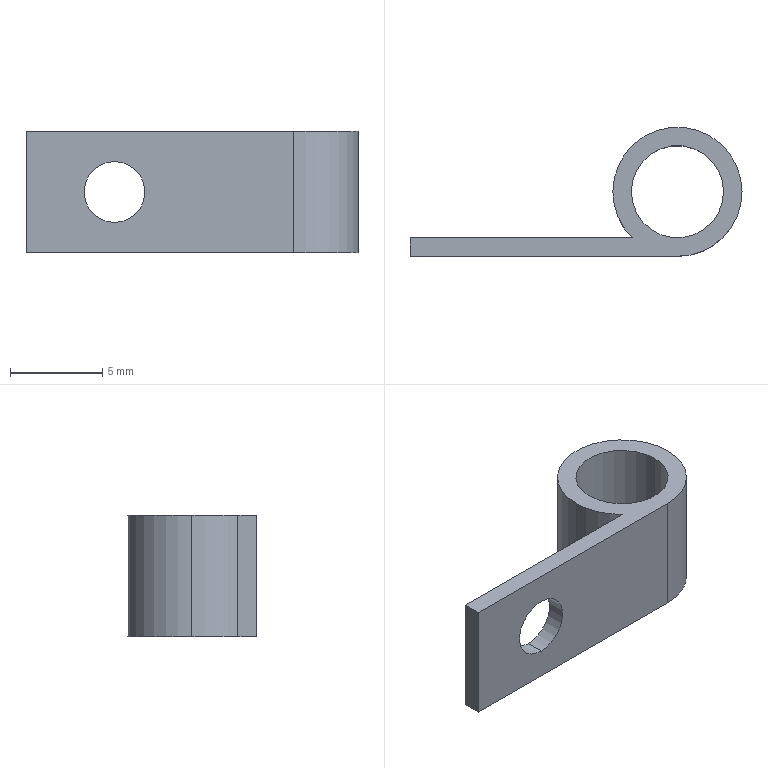Part | SolidWorks | features Extrusion 1, ICE 1 | 1 solid | 12 faces | box 18 x 7 x 6.6 mm | volume 200.425 mm3 | cylinder 7 | plane 5 | commonest cylinder face diameters 7 x3 3.3 x2 5 x2
STEP:
#1=CARTESIAN_POINT('',(4.8,0.,-1.65));
#2=VERTEX_POINT('',#1);
#3=CARTESIAN_POINT('',(4.8,0.,1.65));
#4=VERTEX_POINT('',#3);
#5=CARTESIAN_POINT('',(4.8,0.,0.));
#6=DIRECTION('',(0.,1.,0.));
#7=DIRECTION('',(0.,0.,1.));
#8=AXIS2_PLACEMENT_3D('',#5,#6,#7);
#9=CIRCLE('',#8,1.65);
#10=EDGE_CURVE('',#2,#4,#9,.T.);
#11=ORIENTED_EDGE('',*,*,#10,.F.);
#12=CARTESIAN_POINT('',(4.8,1.,-1.65));
#13=VERTEX_POINT('',#12);
#14=CARTESIAN_POINT('',(4.8,-5.6,-1.65));
#15=DIRECTION('',(0.,1.,0.));
#16=VECTOR('',#15,1000.);
#17=LINE('',#14,#16);
#18=EDGE_CURVE('',#2,#13,#17,.T.);
#19=ORIENTED_EDGE('',*,*,#18,.T.);
#20=CARTESIAN_POINT('',(4.8,1.,1.65));
#21=VERTEX_POINT('',#20);
#22=CARTESIAN_POINT('',(4.8,1.,0.));
#23=DIRECTION('',(0.,1.,0.));
#24=DIRECTION('',(0.,0.,1.));
#25=AXIS2_PLACEMENT_3D('',#22,#23,#24);
#26=CIRCLE('',#25,1.65);
#27=EDGE_CURVE('',#13,#21,#26,.T.);
#28=ORIENTED_EDGE('',*,*,#27,.T.);
#29=CARTESIAN_POINT('',(4.8,-5.6,1.65));
#30=DIRECTION('',(0.,1.,0.));
#31=VECTOR('',#30,1000.);
#32=LINE('',#29,#31);
#33=EDGE_CURVE('',#4,#21,#32,.T.);
#34=ORIENTED_EDGE('',*,*,#33,.F.);
#35=EDGE_LOOP('',(#11,#19,#28,#34));
#36=FACE_OUTER_BOUND('',#35,.T.);
#37=CARTESIAN_POINT('',(4.8,-5.6,0.));
#38=DIRECTION('',(0.,1.,0.));
#39=DIRECTION('',(0.,0.,1.));
#40=AXIS2_PLACEMENT_3D('',#37,#38,#39);
#41=CYLINDRICAL_SURFACE('',#40,1.65);
#42=ADVANCED_FACE('',(#36),#41,.F.);
#43=CARTESIAN_POINT('',(12.,3.5,3.3));
#44=VERTEX_POINT('',#43);
#45=CARTESIAN_POINT('',(17.,3.5,3.3));
#46=VERTEX_POINT('',#45);
#47=CARTESIAN_POINT('',(14.5,3.5,3.3));
#48=DIRECTION('',(0.,0.,1.));
#49=DIRECTION('',(1.,0.,0.));
#50=AXIS2_PLACEMENT_3D('',#47,#48,#49);
#51=CIRCLE('',#50,2.5);
#52=EDGE_CURVE('',#44,#46,#51,.T.);
#53=ORIENTED_EDGE('',*,*,#52,.T.);
#54=CARTESIAN_POINT('',(17.,3.5,-3.3));
#55=VERTEX_POINT('',#54);
#56=CARTESIAN_POINT('',(17.,3.5,3.3));
#57=DIRECTION('',(0.,0.,-1.));
#58=VECTOR('',#57,1000.);
#59=LINE('',#56,#58);
#60=EDGE_CURVE('',#46,#55,#59,.T.);
#61=ORIENTED_EDGE('',*,*,#60,.T.);
#62=CARTESIAN_POINT('',(12.,3.5,-3.3));
#63=VERTEX_POINT('',#62);
#64=CARTESIAN_POINT('',(14.5,3.5,-3.3));
#65=DIRECTION('',(0.,0.,1.));
#66=DIRECTION('',(1.,0.,0.));
#67=AXIS2_PLACEMENT_3D('',#64,#65,#66);
#68=CIRCLE('',#67,2.5);
#69=EDGE_CURVE('',#63,#55,#68,.T.);
#70=ORIENTED_EDGE('',*,*,#69,.F.);
#71=CARTESIAN_POINT('',(12.,3.5,3.3));
#72=DIRECTION('',(0.,0.,-1.));
#73=VECTOR('',#72,1000.);
#74=LINE('',#71,#73);
#75=EDGE_CURVE('',#44,#63,#74,.T.);
#76=ORIENTED_EDGE('',*,*,#75,.F.);
#77=EDGE_LOOP('',(#53,#61,#70,#76));
#78=FACE_OUTER_BOUND('',#77,.T.);
#79=CARTESIAN_POINT('',(14.5,3.5,3.3));
#80=DIRECTION('',(0.,0.,-1.));
#81=DIRECTION('',(-1.,0.,0.));
#82=AXIS2_PLACEMENT_3D('',#79,#80,#81);
#83=CYLINDRICAL_SURFACE('',#82,2.5);
#84=ADVANCED_FACE('',(#78),#83,.F.);
#85=CARTESIAN_POINT('',(18.,3.5,3.3));
#86=VERTEX_POINT('',#85);
#87=CARTESIAN_POINT('',(11.,3.5,3.3));
#88=VERTEX_POINT('',#87);
#89=CARTESIAN_POINT('',(14.5,3.5,3.3));
#90=DIRECTION('',(0.,0.,1.));
#91=DIRECTION('',(1.,0.,0.));
#92=AXIS2_PLACEMENT_3D('',#89,#90,#91);
#93=CIRCLE('',#92,3.5);
#94=EDGE_CURVE('',#86,#88,#93,.T.);
#95=ORIENTED_EDGE('',*,*,#94,.F.);
#96=CARTESIAN_POINT('',(18.,3.5,-3.3));
#97=VERTEX_POINT('',#96);
#98=CARTESIAN_POINT('',(18.,3.5,3.3));
#99=DIRECTION('',(0.,0.,-1.));
#100=VECTOR('',#99,1000.);
#101=LINE('',#98,#100);
#102=EDGE_CURVE('',#86,#97,#101,.T.);
#103=ORIENTED_EDGE('',*,*,#102,.T.);
#104=CARTESIAN_POINT('',(11.,3.5,-3.3));
#105=VERTEX_POINT('',#104);
#106=CARTESIAN_POINT('',(14.5,3.5,-3.3));
#107=DIRECTION('',(0.,0.,1.));
#108=DIRECTION('',(1.,0.,0.));
#109=AXIS2_PLACEMENT_3D('',#106,#107,#108);
#110=CIRCLE('',#109,3.5);
#111=EDGE_CURVE('',#97,#105,#110,.T.);
#112=ORIENTED_EDGE('',*,*,#111,.T.);
#113=CARTESIAN_POINT('',(11.,3.5,3.3));
#114=DIRECTION('',(0.,0.,-1.));
#115=VECTOR('',#114,1000.);
#116=LINE('',#113,#115);
#117=EDGE_CURVE('',#88,#105,#116,.T.);
#118=ORIENTED_EDGE('',*,*,#117,.F.);
#119=EDGE_LOOP('',(#95,#103,#112,#118));
#120=FACE_OUTER_BOUND('',#119,.T.);
#121=CARTESIAN_POINT('',(14.5,3.5,3.3));
#122=DIRECTION('',(0.,0.,-1.));
#123=DIRECTION('',(-1.,0.,0.));
#124=AXIS2_PLACEMENT_3D('',#121,#122,#123);
#125=CYLINDRICAL_SURFACE('',#124,3.5);
#126=ADVANCED_FACE('',(#120),#125,.T.);
#127=CARTESIAN_POINT('',(12.051,1.,3.3));
#128=VERTEX_POINT('',#127);
#129=CARTESIAN_POINT('',(14.5,3.5,3.3));
#130=DIRECTION('',(0.,0.,1.));
#131=DIRECTION('',(1.,0.,0.));
#132=AXIS2_PLACEMENT_3D('',#129,#130,#131);
#133=CIRCLE('',#132,3.5);
#134=EDGE_CURVE('',#88,#128,#133,.T.);
#135=ORIENTED_EDGE('',*,*,#134,.F.);
#136=ORIENTED_EDGE('',*,*,#117,.T.);
#137=CARTESIAN_POINT('',(12.051,1.,-3.3));
#138=VERTEX_POINT('',#137);
#139=CARTESIAN_POINT('',(14.5,3.5,-3.3));
#140=DIRECTION('',(0.,0.,1.));
#141=DIRECTION('',(1.,0.,0.));
#142=AXIS2_PLACEMENT_3D('',#139,#140,#141);
#143=CIRCLE('',#142,3.5);
#144=EDGE_CURVE('',#105,#138,#143,.T.);
#145=ORIENTED_EDGE('',*,*,#144,.T.);
#146=CARTESIAN_POINT('',(12.051,1.,3.3));
#147=DIRECTION('',(0.,0.,-1.));
#148=VECTOR('',#147,1000.);
#149=LINE('',#146,#148);
#150=EDGE_CURVE('',#128,#138,#149,.T.);
#151=ORIENTED_EDGE('',*,*,#150,.F.);
#152=EDGE_LOOP('',(#135,#136,#145,#151));
#153=FACE_OUTER_BOUND('',#152,.T.);
#154=CARTESIAN_POINT('',(14.5,3.5,3.3));
#155=DIRECTION('',(0.,0.,-1.));
#156=DIRECTION('',(-1.,0.,0.));
#157=AXIS2_PLACEMENT_3D('',#154,#155,#156);
#158=CYLINDRICAL_SURFACE('',#157,3.5);
#159=ADVANCED_FACE('',(#153),#158,.T.);
#160=ORIENTED_EDGE('',*,*,#102,.F.);
#161=CARTESIAN_POINT('',(14.5,0.,3.3));
#162=VERTEX_POINT('',#161);
#163=CARTESIAN_POINT('',(14.5,3.5,3.3));
#164=DIRECTION('',(0.,0.,1.));
#165=DIRECTION('',(1.,0.,0.));
#166=AXIS2_PLACEMENT_3D('',#163,#164,#165);
#167=CIRCLE('',#166,3.5);
#168=EDGE_CURVE('',#162,#86,#167,.T.);
#169=ORIENTED_EDGE('',*,*,#168,.F.);
#170=CARTESIAN_POINT('',(14.5,0.,-3.3));
#171=VERTEX_POINT('',#170);
#172=CARTESIAN_POINT('',(14.5,0.,3.3));
#173=DIRECTION('',(0.,0.,-1.));
#174=VECTOR('',#173,1000.);
#175=LINE('',#172,#174);
#176=EDGE_CURVE('',#162,#171,#175,.T.);
#177=ORIENTED_EDGE('',*,*,#176,.T.);
#178=CARTESIAN_POINT('',(14.5,3.5,-3.3));
#179=DIRECTION('',(0.,0.,1.));
#180=DIRECTION('',(1.,0.,0.));
#181=AXIS2_PLACEMENT_3D('',#178,#179,#180);
#182=CIRCLE('',#181,3.5);
#183=EDGE_CURVE('',#171,#97,#182,.T.);
#184=ORIENTED_EDGE('',*,*,#183,.T.);
#185=EDGE_LOOP('',(#160,#169,#177,#184));
#186=FACE_OUTER_BOUND('',#185,.T.);
#187=CARTESIAN_POINT('',(14.5,3.5,3.3));
#188=DIRECTION('',(0.,0.,-1.));
#189=DIRECTION('',(-1.,0.,0.));
#190=AXIS2_PLACEMENT_3D('',#187,#188,#189);
#191=CYLINDRICAL_SURFACE('',#190,3.5);
#192=ADVANCED_FACE('',(#186),#191,.T.);
#193=CARTESIAN_POINT('',(4.8,1.,0.));
#194=DIRECTION('',(0.,1.,0.));
#195=DIRECTION('',(0.,0.,1.));
#196=AXIS2_PLACEMENT_3D('',#193,#194,#195);
#197=CIRCLE('',#196,1.65);
#198=EDGE_CURVE('',#21,#13,#197,.T.);
#199=ORIENTED_EDGE('',*,*,#198,.F.);
#200=ORIENTED_EDGE('',*,*,#27,.F.);
#201=EDGE_LOOP('',(#199,#200));
#202=FACE_BOUND('',#201,.T.);
#203=CARTESIAN_POINT('',(0.,1.,-3.3));
#204=VERTEX_POINT('',#203);
#205=CARTESIAN_POINT('',(0.,1.,-3.3));
#206=DIRECTION('',(1.,0.,0.));
#207=VECTOR('',#206,1000.);
#208=LINE('',#205,#207);
#209=EDGE_CURVE('',#204,#138,#208,.T.);
#210=ORIENTED_EDGE('',*,*,#209,.F.);
#211=CARTESIAN_POINT('',(0.,1.,3.3));
#212=VERTEX_POINT('',#211);
#213=CARTESIAN_POINT('',(0.,1.,3.3));
#214=DIRECTION('',(0.,0.,-1.));
#215=VECTOR('',#214,1000.);
#216=LINE('',#213,#215);
#217=EDGE_CURVE('',#212,#204,#216,.T.);
#218=ORIENTED_EDGE('',*,*,#217,.F.);
#219=CARTESIAN_POINT('',(0.,1.,3.3));
#220=DIRECTION('',(1.,0.,0.));
#221=VECTOR('',#220,1000.);
#222=LINE('',#219,#221);
#223=EDGE_CURVE('',#212,#128,#222,.T.);
#224=ORIENTED_EDGE('',*,*,#223,.T.);
#225=ORIENTED_EDGE('',*,*,#150,.T.);
#226=EDGE_LOOP('',(#210,#218,#224,#225));
#227=FACE_OUTER_BOUND('',#226,.T.);
#228=CARTESIAN_POINT('',(0.,1.,3.3));
#229=DIRECTION('',(0.,1.,0.));
#230=DIRECTION('',(0.,0.,1.));
#231=AXIS2_PLACEMENT_3D('',#228,#229,#230);
#232=PLANE('',#231);
#233=ADVANCED_FACE('',(#202,#227),#232,.T.);
#234=CARTESIAN_POINT('',(0.,0.,-3.3));
#235=VERTEX_POINT('',#234);
#236=CARTESIAN_POINT('',(0.,0.,-3.3));
#237=DIRECTION('',(0.,-1.,0.));
#238=VECTOR('',#237,1000.);
#239=LINE('',#236,#238);
#240=EDGE_CURVE('',#204,#235,#239,.T.);
#241=ORIENTED_EDGE('',*,*,#240,.T.);
#242=CARTESIAN_POINT('',(0.,0.,3.3));
#243=VERTEX_POINT('',#242);
#244=CARTESIAN_POINT('',(0.,0.,3.3));
#245=DIRECTION('',(0.,0.,-1.));
#246=VECTOR('',#245,1000.);
#247=LINE('',#244,#246);
#248=EDGE_CURVE('',#243,#235,#247,.T.);
#249=ORIENTED_EDGE('',*,*,#248,.F.);
#250=CARTESIAN_POINT('',(0.,0.,3.3));
#251=DIRECTION('',(0.,-1.,0.));
#252=VECTOR('',#251,1000.);
#253=LINE('',#250,#252);
#254=EDGE_CURVE('',#212,#243,#253,.T.);
#255=ORIENTED_EDGE('',*,*,#254,.F.);
#256=ORIENTED_EDGE('',*,*,#217,.T.);
#257=EDGE_LOOP('',(#241,#249,#255,#256));
#258=FACE_OUTER_BOUND('',#257,.T.);
#259=CARTESIAN_POINT('',(0.,0.,3.3));
#260=DIRECTION('',(1.,0.,0.));
#261=DIRECTION('',(0.,0.,-1.));
#262=AXIS2_PLACEMENT_3D('',#259,#260,#261);
#263=PLANE('',#262);
#264=ADVANCED_FACE('',(#258),#263,.F.);
#265=ORIENTED_EDGE('',*,*,#60,.F.);
#266=CARTESIAN_POINT('',(14.5,3.5,3.3));
#267=DIRECTION('',(0.,0.,1.));
#268=DIRECTION('',(1.,0.,0.));
#269=AXIS2_PLACEMENT_3D('',#266,#267,#268);
#270=CIRCLE('',#269,2.5);
#271=EDGE_CURVE('',#46,#44,#270,.T.);
#272=ORIENTED_EDGE('',*,*,#271,.T.);
#273=ORIENTED_EDGE('',*,*,#75,.T.);
#274=CARTESIAN_POINT('',(14.5,3.5,-3.3));
#275=DIRECTION('',(0.,0.,1.));
#276=DIRECTION('',(1.,0.,0.));
#277=AXIS2_PLACEMENT_3D('',#274,#275,#276);
#278=CIRCLE('',#277,2.5);
#279=EDGE_CURVE('',#55,#63,#278,.T.);
#280=ORIENTED_EDGE('',*,*,#279,.F.);
#281=EDGE_LOOP('',(#265,#272,#273,#280));
#282=FACE_OUTER_BOUND('',#281,.T.);
#283=CARTESIAN_POINT('',(14.5,3.5,3.3));
#284=DIRECTION('',(0.,0.,-1.));
#285=DIRECTION('',(-1.,0.,0.));
#286=AXIS2_PLACEMENT_3D('',#283,#284,#285);
#287=CYLINDRICAL_SURFACE('',#286,2.5);
#288=ADVANCED_FACE('',(#282),#287,.F.);
#289=CARTESIAN_POINT('',(4.8,0.,0.));
#290=DIRECTION('',(0.,1.,0.));
#291=DIRECTION('',(0.,0.,1.));
#292=AXIS2_PLACEMENT_3D('',#289,#290,#291);
#293=CIRCLE('',#292,1.65);
#294=EDGE_CURVE('',#4,#2,#293,.T.);
#295=ORIENTED_EDGE('',*,*,#294,.T.);
#296=ORIENTED_EDGE('',*,*,#10,.T.);
#297=EDGE_LOOP('',(#295,#296));
#298=FACE_BOUND('',#297,.T.);
#299=CARTESIAN_POINT('',(0.,0.,-3.3));
#300=DIRECTION('',(1.,0.,0.));
#301=VECTOR('',#300,1000.);
#302=LINE('',#299,#301);
#303=EDGE_CURVE('',#235,#171,#302,.T.);
#304=ORIENTED_EDGE('',*,*,#303,.T.);
#305=ORIENTED_EDGE('',*,*,#176,.F.);
#306=CARTESIAN_POINT('',(0.,0.,3.3));
#307=DIRECTION('',(1.,0.,0.));
#308=VECTOR('',#307,1000.);
#309=LINE('',#306,#308);
#310=EDGE_CURVE('',#243,#162,#309,.T.);
#311=ORIENTED_EDGE('',*,*,#310,.F.);
#312=ORIENTED_EDGE('',*,*,#248,.T.);
#313=EDGE_LOOP('',(#304,#305,#311,#312));
#314=FACE_OUTER_BOUND('',#313,.T.);
#315=CARTESIAN_POINT('',(0.,0.,3.3));
#316=DIRECTION('',(0.,1.,0.));
#317=DIRECTION('',(0.,0.,1.));
#318=AXIS2_PLACEMENT_3D('',#315,#316,#317);
#319=PLANE('',#318);
#320=ADVANCED_FACE('',(#298,#314),#319,.F.);
#321=ORIENTED_EDGE('',*,*,#52,.F.);
#322=ORIENTED_EDGE('',*,*,#271,.F.);
#323=EDGE_LOOP('',(#321,#322));
#324=FACE_BOUND('',#323,.T.);
#325=ORIENTED_EDGE('',*,*,#168,.T.);
#326=ORIENTED_EDGE('',*,*,#94,.T.);
#327=ORIENTED_EDGE('',*,*,#134,.T.);
#328=ORIENTED_EDGE('',*,*,#223,.F.);
#329=ORIENTED_EDGE('',*,*,#254,.T.);
#330=ORIENTED_EDGE('',*,*,#310,.T.);
#331=EDGE_LOOP('',(#325,#326,#327,#328,#329,#330));
#332=FACE_OUTER_BOUND('',#331,.T.);
#333=CARTESIAN_POINT('',(0.,0.,3.3));
#334=DIRECTION('',(0.,0.,1.));
#335=DIRECTION('',(1.,0.,0.));
#336=AXIS2_PLACEMENT_3D('',#333,#334,#335);
#337=PLANE('',#336);
#338=ADVANCED_FACE('',(#324,#332),#337,.T.);
#339=ORIENTED_EDGE('',*,*,#69,.T.);
#340=ORIENTED_EDGE('',*,*,#279,.T.);
#341=EDGE_LOOP('',(#339,#340));
#342=FACE_BOUND('',#341,.T.);
#343=ORIENTED_EDGE('',*,*,#183,.F.);
#344=ORIENTED_EDGE('',*,*,#303,.F.);
#345=ORIENTED_EDGE('',*,*,#240,.F.);
#346=ORIENTED_EDGE('',*,*,#209,.T.);
#347=ORIENTED_EDGE('',*,*,#144,.F.);
#348=ORIENTED_EDGE('',*,*,#111,.F.);
#349=EDGE_LOOP('',(#343,#344,#345,#346,#347,#348));
#350=FACE_OUTER_BOUND('',#349,.T.);
#351=CARTESIAN_POINT('',(0.,0.,-3.3));
#352=DIRECTION('',(0.,0.,1.));
#353=DIRECTION('',(1.,0.,0.));
#354=AXIS2_PLACEMENT_3D('',#351,#352,#353);
#355=PLANE('',#354);
#356=ADVANCED_FACE('',(#342,#350),#355,.F.);
#357=ORIENTED_EDGE('',*,*,#18,.F.);
#358=ORIENTED_EDGE('',*,*,#294,.F.);
#359=ORIENTED_EDGE('',*,*,#33,.T.);
#360=ORIENTED_EDGE('',*,*,#198,.T.);
#361=EDGE_LOOP('',(#357,#358,#359,#360));
#362=FACE_OUTER_BOUND('',#361,.T.);
#363=CARTESIAN_POINT('',(4.8,-5.6,0.));
#364=DIRECTION('',(0.,1.,0.));
#365=DIRECTION('',(0.,0.,1.));
#366=AXIS2_PLACEMENT_3D('',#363,#364,#365);
#367=CYLINDRICAL_SURFACE('',#366,1.65);
#368=ADVANCED_FACE('',(#362),#367,.F.);
#369=CLOSED_SHELL('',(#42,#84,#126,#159,#192,#233,#264,#288,#320,#338,#356,#368));
#370=MANIFOLD_SOLID_BREP('',#369);
#371=CARTESIAN_POINT('',(0.,0.,0.));
#372=DIRECTION('',(0.,0.,1.));
#373=DIRECTION('',(1.,0.,0.));
#374=AXIS2_PLACEMENT_3D('',#371,#372,#373);
#375=(LENGTH_UNIT()NAMED_UNIT(*)SI_UNIT(.MILLI.,.METRE.));
#376=UNCERTAINTY_MEASURE_WITH_UNIT(LENGTH_MEASURE(0.00001),#375,'','');
#377=(NAMED_UNIT(*)PLANE_ANGLE_UNIT()SI_UNIT($,.RADIAN.));
#378=(NAMED_UNIT(*)SI_UNIT($,.STERADIAN.)SOLID_ANGLE_UNIT());
#379=(GEOMETRIC_REPRESENTATION_CONTEXT(3)GLOBAL_UNCERTAINTY_ASSIGNED_CONTEXT((#376))GLOBAL_UNIT_ASSIGNED_CONTEXT((#375,#377,#378))REPRESENTATION_CONTEXT('',''));
#380=ADVANCED_BREP_SHAPE_REPRESENTATION('',(#370,#374),#379);